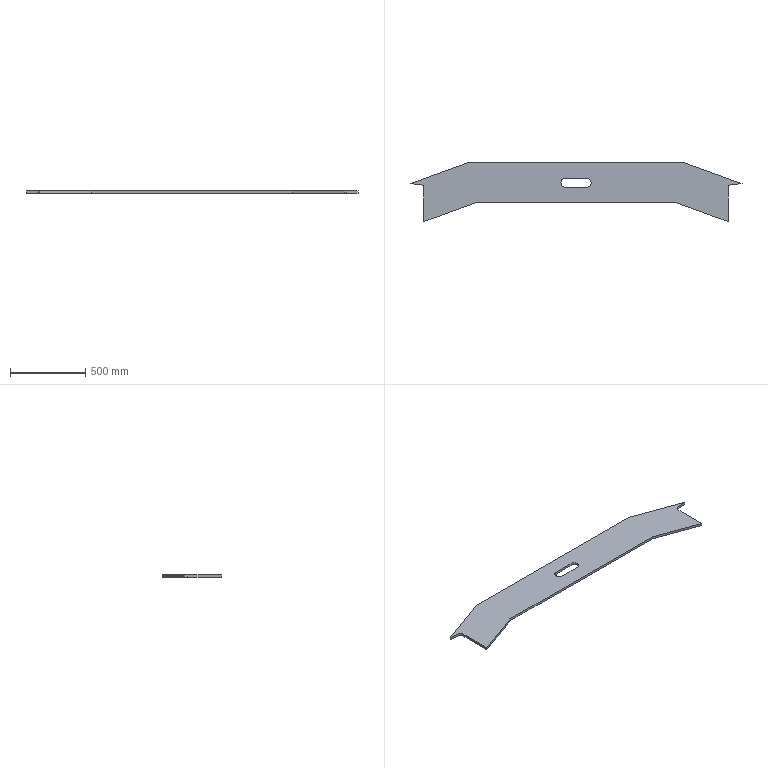Part | SolidWorks | features ICE 2, Fillet 1, FlatPattern 1, SMBaseFlange 1, SheetMetal 1 | 1 solid | 19 faces | box 2205 x 392.571 x 16 mm | volume 8722850 mm3 | plane 14 | cylinder 5 | commonest cylinder face diameters 60 x3 40 x2
STEP:
#1=CARTESIAN_POINT('',(-100.,-134.,0.));
#2=VERTEX_POINT('',#1);
#3=CARTESIAN_POINT('',(-70.,-104.,0.));
#4=VERTEX_POINT('',#3);
#5=CARTESIAN_POINT('',(-70.,-134.,0.));
#6=DIRECTION('',(0.,0.,-1.));
#7=DIRECTION('',(-1.,0.,0.));
#8=AXIS2_PLACEMENT_3D('',#5,#6,#7);
#9=CIRCLE('',#8,30.);
#10=EDGE_CURVE('',#2,#4,#9,.T.);
#11=ORIENTED_EDGE('',*,*,#10,.F.);
#12=CARTESIAN_POINT('',(-100.,-134.,-16.));
#13=VERTEX_POINT('',#12);
#14=CARTESIAN_POINT('',(-100.,-134.,0.));
#15=DIRECTION('',(0.,0.,-1.));
#16=VECTOR('',#15,1000.);
#17=LINE('',#14,#16);
#18=EDGE_CURVE('',#2,#13,#17,.T.);
#19=ORIENTED_EDGE('',*,*,#18,.T.);
#20=CARTESIAN_POINT('',(-70.,-104.,-16.));
#21=VERTEX_POINT('',#20);
#22=CARTESIAN_POINT('',(-70.,-134.,-16.));
#23=DIRECTION('',(0.,0.,-1.));
#24=DIRECTION('',(-1.,0.,0.));
#25=AXIS2_PLACEMENT_3D('',#22,#23,#24);
#26=CIRCLE('',#25,30.);
#27=EDGE_CURVE('',#13,#21,#26,.T.);
#28=ORIENTED_EDGE('',*,*,#27,.T.);
#29=CARTESIAN_POINT('',(-70.,-104.,0.));
#30=DIRECTION('',(0.,0.,-1.));
#31=VECTOR('',#30,1000.);
#32=LINE('',#29,#31);
#33=EDGE_CURVE('',#4,#21,#32,.T.);
#34=ORIENTED_EDGE('',*,*,#33,.F.);
#35=EDGE_LOOP('',(#11,#19,#28,#34));
#36=FACE_OUTER_BOUND('',#35,.T.);
#37=CARTESIAN_POINT('',(-70.,-134.,0.));
#38=DIRECTION('',(0.,0.,-1.));
#39=DIRECTION('',(-1.,0.,0.));
#40=AXIS2_PLACEMENT_3D('',#37,#38,#39);
#41=CYLINDRICAL_SURFACE('',#40,30.);
#42=ADVANCED_FACE('',(#36),#41,.F.);
#43=CARTESIAN_POINT('',(715.,0.,0.));
#44=VERTEX_POINT('',#43);
#45=CARTESIAN_POINT('',(-715.,0.,0.));
#46=VERTEX_POINT('',#45);
#47=CARTESIAN_POINT('',(-715.,0.,0.));
#48=DIRECTION('',(-1.,0.,0.));
#49=VECTOR('',#48,1000.);
#50=LINE('',#47,#49);
#51=EDGE_CURVE('',#44,#46,#50,.T.);
#52=ORIENTED_EDGE('',*,*,#51,.F.);
#53=CARTESIAN_POINT('',(715.,0.,-16.));
#54=VERTEX_POINT('',#53);
#55=CARTESIAN_POINT('',(715.,0.,-16.));
#56=DIRECTION('',(0.,0.,1.));
#57=VECTOR('',#56,1000.);
#58=LINE('',#55,#57);
#59=EDGE_CURVE('',#54,#44,#58,.T.);
#60=ORIENTED_EDGE('',*,*,#59,.F.);
#61=CARTESIAN_POINT('',(-715.,0.,-16.));
#62=VERTEX_POINT('',#61);
#63=CARTESIAN_POINT('',(-715.,0.,-16.));
#64=DIRECTION('',(-1.,0.,0.));
#65=VECTOR('',#64,1000.);
#66=LINE('',#63,#65);
#67=EDGE_CURVE('',#54,#62,#66,.T.);
#68=ORIENTED_EDGE('',*,*,#67,.T.);
#69=CARTESIAN_POINT('',(-715.,0.,-16.));
#70=DIRECTION('',(0.,0.,1.));
#71=VECTOR('',#70,1000.);
#72=LINE('',#69,#71);
#73=EDGE_CURVE('',#62,#46,#72,.T.);
#74=ORIENTED_EDGE('',*,*,#73,.T.);
#75=EDGE_LOOP('',(#52,#60,#68,#74));
#76=FACE_OUTER_BOUND('',#75,.T.);
#77=CARTESIAN_POINT('',(-715.,0.,-16.));
#78=DIRECTION('',(0.,1.,0.));
#79=DIRECTION('',(0.,0.,1.));
#80=AXIS2_PLACEMENT_3D('',#77,#78,#79);
#81=PLANE('',#80);
#82=ADVANCED_FACE('',(#76),#81,.T.);
#83=CARTESIAN_POINT('',(1102.619,-141.082,-16.));
#84=VERTEX_POINT('',#83);
#85=CARTESIAN_POINT('',(1102.619,-141.082,0.));
#86=VERTEX_POINT('',#85);
#87=CARTESIAN_POINT('',(1102.619,-141.082,-16.));
#88=DIRECTION('',(0.,0.,1.));
#89=VECTOR('',#88,1000.);
#90=LINE('',#87,#89);
#91=EDGE_CURVE('',#84,#86,#90,.T.);
#92=ORIENTED_EDGE('',*,*,#91,.F.);
#93=CARTESIAN_POINT('',(715.,0.,-16.));
#94=DIRECTION('',(-0.9397,0.342,0.));
#95=VECTOR('',#94,1000.);
#96=LINE('',#93,#95);
#97=EDGE_CURVE('',#84,#54,#96,.T.);
#98=ORIENTED_EDGE('',*,*,#97,.T.);
#99=ORIENTED_EDGE('',*,*,#59,.T.);
#100=CARTESIAN_POINT('',(715.,0.,0.));
#101=DIRECTION('',(-0.9397,0.342,0.));
#102=VECTOR('',#101,1000.);
#103=LINE('',#100,#102);
#104=EDGE_CURVE('',#86,#44,#103,.T.);
#105=ORIENTED_EDGE('',*,*,#104,.F.);
#106=EDGE_LOOP('',(#92,#98,#99,#105));
#107=FACE_OUTER_BOUND('',#106,.T.);
#108=CARTESIAN_POINT('',(715.,0.,-16.));
#109=DIRECTION('',(0.342,0.9397,0.));
#110=DIRECTION('',(-0.9397,0.342,0.));
#111=AXIS2_PLACEMENT_3D('',#108,#109,#110);
#112=PLANE('',#111);
#113=ADVANCED_FACE('',(#107),#112,.T.);
#114=CARTESIAN_POINT('',(1010.,-392.571,0.));
#115=VERTEX_POINT('',#114);
#116=CARTESIAN_POINT('',(1010.,-392.571,-16.));
#117=VERTEX_POINT('',#116);
#118=CARTESIAN_POINT('',(1010.,-392.571,-16.));
#119=DIRECTION('',(0.,0.,-1.));
#120=VECTOR('',#119,1000.);
#121=LINE('',#118,#120);
#122=EDGE_CURVE('',#115,#117,#121,.T.);
#123=ORIENTED_EDGE('',*,*,#122,.F.);
#124=CARTESIAN_POINT('',(667.744,-268.,0.));
#125=VERTEX_POINT('',#124);
#126=CARTESIAN_POINT('',(667.744,-268.,0.));
#127=DIRECTION('',(0.9397,-0.342,0.));
#128=VECTOR('',#127,1000.);
#129=LINE('',#126,#128);
#130=EDGE_CURVE('',#125,#115,#129,.T.);
#131=ORIENTED_EDGE('',*,*,#130,.F.);
#132=CARTESIAN_POINT('',(667.744,-268.,-16.));
#133=VERTEX_POINT('',#132);
#134=CARTESIAN_POINT('',(667.744,-268.,-16.));
#135=DIRECTION('',(0.,0.,1.));
#136=VECTOR('',#135,1000.);
#137=LINE('',#134,#136);
#138=EDGE_CURVE('',#133,#125,#137,.T.);
#139=ORIENTED_EDGE('',*,*,#138,.F.);
#140=CARTESIAN_POINT('',(667.744,-268.,-16.));
#141=DIRECTION('',(0.9397,-0.342,0.));
#142=VECTOR('',#141,1000.);
#143=LINE('',#140,#142);
#144=EDGE_CURVE('',#133,#117,#143,.T.);
#145=ORIENTED_EDGE('',*,*,#144,.T.);
#146=EDGE_LOOP('',(#123,#131,#139,#145));
#147=FACE_OUTER_BOUND('',#146,.T.);
#148=CARTESIAN_POINT('',(667.744,-268.,-16.));
#149=DIRECTION('',(-0.342,-0.9397,0.));
#150=DIRECTION('',(0.9397,-0.342,0.));
#151=AXIS2_PLACEMENT_3D('',#148,#149,#150);
#152=PLANE('',#151);
#153=ADVANCED_FACE('',(#147),#152,.T.);
#154=CARTESIAN_POINT('',(-667.744,-268.,0.));
#155=VERTEX_POINT('',#154);
#156=CARTESIAN_POINT('',(-667.744,-268.,0.));
#157=DIRECTION('',(1.,0.,0.));
#158=VECTOR('',#157,1000.);
#159=LINE('',#156,#158);
#160=EDGE_CURVE('',#155,#125,#159,.T.);
#161=ORIENTED_EDGE('',*,*,#160,.F.);
#162=CARTESIAN_POINT('',(-667.744,-268.,-16.));
#163=VERTEX_POINT('',#162);
#164=CARTESIAN_POINT('',(-667.744,-268.,-16.));
#165=DIRECTION('',(0.,0.,1.));
#166=VECTOR('',#165,1000.);
#167=LINE('',#164,#166);
#168=EDGE_CURVE('',#163,#155,#167,.T.);
#169=ORIENTED_EDGE('',*,*,#168,.F.);
#170=CARTESIAN_POINT('',(-667.744,-268.,-16.));
#171=DIRECTION('',(1.,0.,0.));
#172=VECTOR('',#171,1000.);
#173=LINE('',#170,#172);
#174=EDGE_CURVE('',#163,#133,#173,.T.);
#175=ORIENTED_EDGE('',*,*,#174,.T.);
#176=ORIENTED_EDGE('',*,*,#138,.T.);
#177=EDGE_LOOP('',(#161,#169,#175,#176));
#178=FACE_OUTER_BOUND('',#177,.T.);
#179=CARTESIAN_POINT('',(-667.744,-268.,-16.));
#180=DIRECTION('',(0.,-1.,0.));
#181=DIRECTION('',(0.,0.,-1.));
#182=AXIS2_PLACEMENT_3D('',#179,#180,#181);
#183=PLANE('',#182);
#184=ADVANCED_FACE('',(#178),#183,.T.);
#185=CARTESIAN_POINT('',(-1010.,-392.571,-16.));
#186=VERTEX_POINT('',#185);
#187=CARTESIAN_POINT('',(-1010.,-392.571,0.));
#188=VERTEX_POINT('',#187);
#189=CARTESIAN_POINT('',(-1010.,-392.571,-16.));
#190=DIRECTION('',(0.,0.,1.));
#191=VECTOR('',#190,1000.);
#192=LINE('',#189,#191);
#193=EDGE_CURVE('',#186,#188,#192,.T.);
#194=ORIENTED_EDGE('',*,*,#193,.F.);
#195=CARTESIAN_POINT('',(-667.744,-268.,-16.));
#196=DIRECTION('',(0.9397,0.342,0.));
#197=VECTOR('',#196,1000.);
#198=LINE('',#195,#197);
#199=EDGE_CURVE('',#186,#163,#198,.T.);
#200=ORIENTED_EDGE('',*,*,#199,.T.);
#201=ORIENTED_EDGE('',*,*,#168,.T.);
#202=CARTESIAN_POINT('',(-667.744,-268.,0.));
#203=DIRECTION('',(0.9397,0.342,0.));
#204=VECTOR('',#203,1000.);
#205=LINE('',#202,#204);
#206=EDGE_CURVE('',#188,#155,#205,.T.);
#207=ORIENTED_EDGE('',*,*,#206,.F.);
#208=EDGE_LOOP('',(#194,#200,#201,#207));
#209=FACE_OUTER_BOUND('',#208,.T.);
#210=CARTESIAN_POINT('',(-667.744,-268.,-16.));
#211=DIRECTION('',(0.342,-0.9397,0.));
#212=DIRECTION('',(0.9397,0.342,0.));
#213=AXIS2_PLACEMENT_3D('',#210,#211,#212);
#214=PLANE('',#213);
#215=ADVANCED_FACE('',(#209),#214,.T.);
#216=CARTESIAN_POINT('',(-1102.619,-141.082,0.));
#217=VERTEX_POINT('',#216);
#218=CARTESIAN_POINT('',(-1102.619,-141.082,-16.));
#219=VERTEX_POINT('',#218);
#220=CARTESIAN_POINT('',(-1102.619,-141.082,-16.));
#221=DIRECTION('',(0.,0.,-1.));
#222=VECTOR('',#221,1000.);
#223=LINE('',#220,#222);
#224=EDGE_CURVE('',#217,#219,#223,.T.);
#225=ORIENTED_EDGE('',*,*,#224,.F.);
#226=CARTESIAN_POINT('',(-715.,0.,0.));
#227=DIRECTION('',(-0.9397,-0.342,0.));
#228=VECTOR('',#227,1000.);
#229=LINE('',#226,#228);
#230=EDGE_CURVE('',#46,#217,#229,.T.);
#231=ORIENTED_EDGE('',*,*,#230,.F.);
#232=ORIENTED_EDGE('',*,*,#73,.F.);
#233=CARTESIAN_POINT('',(-715.,0.,-16.));
#234=DIRECTION('',(-0.9397,-0.342,0.));
#235=VECTOR('',#234,1000.);
#236=LINE('',#233,#235);
#237=EDGE_CURVE('',#62,#219,#236,.T.);
#238=ORIENTED_EDGE('',*,*,#237,.T.);
#239=EDGE_LOOP('',(#225,#231,#232,#238));
#240=FACE_OUTER_BOUND('',#239,.T.);
#241=CARTESIAN_POINT('',(-715.,0.,-16.));
#242=DIRECTION('',(-0.342,0.9397,0.));
#243=DIRECTION('',(-0.9397,-0.342,0.));
#244=AXIS2_PLACEMENT_3D('',#241,#242,#243);
#245=PLANE('',#244);
#246=ADVANCED_FACE('',(#240),#245,.T.);
#247=CARTESIAN_POINT('',(70.,-164.,-16.));
#248=VERTEX_POINT('',#247);
#249=CARTESIAN_POINT('',(-70.,-164.,-16.));
#250=VERTEX_POINT('',#249);
#251=CARTESIAN_POINT('',(70.,-164.,-16.));
#252=DIRECTION('',(-1.,0.,0.));
#253=VECTOR('',#252,1000.);
#254=LINE('',#251,#253);
#255=EDGE_CURVE('',#248,#250,#254,.T.);
#256=ORIENTED_EDGE('',*,*,#255,.F.);
#257=CARTESIAN_POINT('',(70.,-104.,-16.));
#258=VERTEX_POINT('',#257);
#259=CARTESIAN_POINT('',(70.,-134.,-16.));
#260=DIRECTION('',(0.,0.,-1.));
#261=DIRECTION('',(-1.,0.,0.));
#262=AXIS2_PLACEMENT_3D('',#259,#260,#261);
#263=CIRCLE('',#262,30.);
#264=EDGE_CURVE('',#258,#248,#263,.T.);
#265=ORIENTED_EDGE('',*,*,#264,.F.);
#266=CARTESIAN_POINT('',(70.,-104.,-16.));
#267=DIRECTION('',(1.,0.,0.));
#268=VECTOR('',#267,1000.);
#269=LINE('',#266,#268);
#270=EDGE_CURVE('',#21,#258,#269,.T.);
#271=ORIENTED_EDGE('',*,*,#270,.F.);
#272=ORIENTED_EDGE('',*,*,#27,.F.);
#273=CARTESIAN_POINT('',(-70.,-134.,-16.));
#274=DIRECTION('',(0.,0.,-1.));
#275=DIRECTION('',(-1.,0.,0.));
#276=AXIS2_PLACEMENT_3D('',#273,#274,#275);
#277=CIRCLE('',#276,30.);
#278=EDGE_CURVE('',#250,#13,#277,.T.);
#279=ORIENTED_EDGE('',*,*,#278,.F.);
#280=EDGE_LOOP('',(#256,#265,#271,#272,#279));
#281=FACE_BOUND('',#280,.T.);
#282=CARTESIAN_POINT('',(-1010.,-168.167,-16.));
#283=VERTEX_POINT('',#282);
#284=CARTESIAN_POINT('',(-1010.,-150.,-16.));
#285=DIRECTION('',(0.,1.,0.));
#286=VECTOR('',#285,1000.);
#287=LINE('',#284,#286);
#288=EDGE_CURVE('',#186,#283,#287,.T.);
#289=ORIENTED_EDGE('',*,*,#288,.T.);
#290=CARTESIAN_POINT('',(-1028.083,-148.259,-16.));
#291=VERTEX_POINT('',#290);
#292=CARTESIAN_POINT('',(-1030.,-168.167,-16.));
#293=DIRECTION('',(0.,0.,1.));
#294=DIRECTION('',(1.,0.,0.));
#295=AXIS2_PLACEMENT_3D('',#292,#293,#294);
#296=CIRCLE('',#295,20.);
#297=EDGE_CURVE('',#283,#291,#296,.T.);
#298=ORIENTED_EDGE('',*,*,#297,.T.);
#299=CARTESIAN_POINT('',(-1310.,-121.113,-16.));
#300=DIRECTION('',(-0.9954,0.09585,0.));
#301=VECTOR('',#300,1000.);
#302=LINE('',#299,#301);
#303=EDGE_CURVE('',#291,#219,#302,.T.);
#304=ORIENTED_EDGE('',*,*,#303,.T.);
#305=ORIENTED_EDGE('',*,*,#237,.F.);
#306=ORIENTED_EDGE('',*,*,#67,.F.);
#307=ORIENTED_EDGE('',*,*,#97,.F.);
#308=CARTESIAN_POINT('',(1028.083,-148.259,-16.));
#309=VERTEX_POINT('',#308);
#310=CARTESIAN_POINT('',(1310.,-121.113,-16.));
#311=DIRECTION('',(-0.9954,-0.09585,0.));
#312=VECTOR('',#311,1000.);
#313=LINE('',#310,#312);
#314=EDGE_CURVE('',#84,#309,#313,.T.);
#315=ORIENTED_EDGE('',*,*,#314,.T.);
#316=CARTESIAN_POINT('',(1010.,-168.167,-16.));
#317=VERTEX_POINT('',#316);
#318=CARTESIAN_POINT('',(1030.,-168.167,-16.));
#319=DIRECTION('',(0.,0.,1.));
#320=DIRECTION('',(1.,0.,0.));
#321=AXIS2_PLACEMENT_3D('',#318,#319,#320);
#322=CIRCLE('',#321,20.);
#323=EDGE_CURVE('',#309,#317,#322,.T.);
#324=ORIENTED_EDGE('',*,*,#323,.T.);
#325=CARTESIAN_POINT('',(1010.,-150.,-16.));
#326=DIRECTION('',(0.,-1.,0.));
#327=VECTOR('',#326,1000.);
#328=LINE('',#325,#327);
#329=EDGE_CURVE('',#317,#117,#328,.T.);
#330=ORIENTED_EDGE('',*,*,#329,.T.);
#331=ORIENTED_EDGE('',*,*,#144,.F.);
#332=ORIENTED_EDGE('',*,*,#174,.F.);
#333=ORIENTED_EDGE('',*,*,#199,.F.);
#334=EDGE_LOOP('',(#289,#298,#304,#305,#306,#307,#315,#324,#330,#331,#332,#333));
#335=FACE_OUTER_BOUND('',#334,.T.);
#336=CARTESIAN_POINT('',(0.,0.,-16.));
#337=DIRECTION('',(0.,0.,1.));
#338=DIRECTION('',(1.,0.,0.));
#339=AXIS2_PLACEMENT_3D('',#336,#337,#338);
#340=PLANE('',#339);
#341=ADVANCED_FACE('',(#281,#335),#340,.F.);
#342=CARTESIAN_POINT('',(70.,-104.,0.));
#343=VERTEX_POINT('',#342);
#344=CARTESIAN_POINT('',(70.,-164.,0.));
#345=VERTEX_POINT('',#344);
#346=CARTESIAN_POINT('',(70.,-134.,0.));
#347=DIRECTION('',(0.,0.,-1.));
#348=DIRECTION('',(-1.,0.,0.));
#349=AXIS2_PLACEMENT_3D('',#346,#347,#348);
#350=CIRCLE('',#349,30.);
#351=EDGE_CURVE('',#343,#345,#350,.T.);
#352=ORIENTED_EDGE('',*,*,#351,.T.);
#353=CARTESIAN_POINT('',(-70.,-164.,0.));
#354=VERTEX_POINT('',#353);
#355=CARTESIAN_POINT('',(70.,-164.,0.));
#356=DIRECTION('',(-1.,0.,0.));
#357=VECTOR('',#356,1000.);
#358=LINE('',#355,#357);
#359=EDGE_CURVE('',#345,#354,#358,.T.);
#360=ORIENTED_EDGE('',*,*,#359,.T.);
#361=CARTESIAN_POINT('',(-70.,-134.,0.));
#362=DIRECTION('',(0.,0.,-1.));
#363=DIRECTION('',(-1.,0.,0.));
#364=AXIS2_PLACEMENT_3D('',#361,#362,#363);
#365=CIRCLE('',#364,30.);
#366=EDGE_CURVE('',#354,#2,#365,.T.);
#367=ORIENTED_EDGE('',*,*,#366,.T.);
#368=ORIENTED_EDGE('',*,*,#10,.T.);
#369=CARTESIAN_POINT('',(70.,-104.,0.));
#370=DIRECTION('',(1.,0.,0.));
#371=VECTOR('',#370,1000.);
#372=LINE('',#369,#371);
#373=EDGE_CURVE('',#4,#343,#372,.T.);
#374=ORIENTED_EDGE('',*,*,#373,.T.);
#375=EDGE_LOOP('',(#352,#360,#367,#368,#374));
#376=FACE_BOUND('',#375,.T.);
#377=CARTESIAN_POINT('',(-1028.083,-148.259,0.));
#378=VERTEX_POINT('',#377);
#379=CARTESIAN_POINT('',(-1310.,-121.113,0.));
#380=DIRECTION('',(-0.9954,0.09585,0.));
#381=VECTOR('',#380,1000.);
#382=LINE('',#379,#381);
#383=EDGE_CURVE('',#378,#217,#382,.T.);
#384=ORIENTED_EDGE('',*,*,#383,.F.);
#385=CARTESIAN_POINT('',(-1010.,-168.167,0.));
#386=VERTEX_POINT('',#385);
#387=CARTESIAN_POINT('',(-1030.,-168.167,0.));
#388=DIRECTION('',(0.,0.,-1.));
#389=DIRECTION('',(1.,0.,0.));
#390=AXIS2_PLACEMENT_3D('',#387,#388,#389);
#391=CIRCLE('',#390,20.);
#392=EDGE_CURVE('',#378,#386,#391,.T.);
#393=ORIENTED_EDGE('',*,*,#392,.T.);
#394=CARTESIAN_POINT('',(-1010.,0.,0.));
#395=DIRECTION('',(0.,1.,0.));
#396=VECTOR('',#395,1000.);
#397=LINE('',#394,#396);
#398=EDGE_CURVE('',#188,#386,#397,.T.);
#399=ORIENTED_EDGE('',*,*,#398,.F.);
#400=ORIENTED_EDGE('',*,*,#206,.T.);
#401=ORIENTED_EDGE('',*,*,#160,.T.);
#402=ORIENTED_EDGE('',*,*,#130,.T.);
#403=CARTESIAN_POINT('',(1010.,-168.167,0.));
#404=VERTEX_POINT('',#403);
#405=CARTESIAN_POINT('',(1010.,-150.,0.));
#406=DIRECTION('',(0.,-1.,0.));
#407=VECTOR('',#406,1000.);
#408=LINE('',#405,#407);
#409=EDGE_CURVE('',#404,#115,#408,.T.);
#410=ORIENTED_EDGE('',*,*,#409,.F.);
#411=CARTESIAN_POINT('',(1028.083,-148.259,0.));
#412=VERTEX_POINT('',#411);
#413=CARTESIAN_POINT('',(1030.,-168.167,0.));
#414=DIRECTION('',(0.,0.,-1.));
#415=DIRECTION('',(1.,0.,0.));
#416=AXIS2_PLACEMENT_3D('',#413,#414,#415);
#417=CIRCLE('',#416,20.);
#418=EDGE_CURVE('',#404,#412,#417,.T.);
#419=ORIENTED_EDGE('',*,*,#418,.T.);
#420=CARTESIAN_POINT('',(23.589,-244.981,0.));
#421=DIRECTION('',(-0.9954,-0.09585,0.));
#422=VECTOR('',#421,1000.);
#423=LINE('',#420,#422);
#424=EDGE_CURVE('',#86,#412,#423,.T.);
#425=ORIENTED_EDGE('',*,*,#424,.F.);
#426=ORIENTED_EDGE('',*,*,#104,.T.);
#427=ORIENTED_EDGE('',*,*,#51,.T.);
#428=ORIENTED_EDGE('',*,*,#230,.T.);
#429=EDGE_LOOP('',(#384,#393,#399,#400,#401,#402,#410,#419,#425,#426,#427,#428));
#430=FACE_OUTER_BOUND('',#429,.T.);
#431=CARTESIAN_POINT('',(0.,0.,0.));
#432=DIRECTION('',(0.,0.,1.));
#433=DIRECTION('',(1.,0.,0.));
#434=AXIS2_PLACEMENT_3D('',#431,#432,#433);
#435=PLANE('',#434);
#436=ADVANCED_FACE('',(#376,#430),#435,.T.);
#437=ORIENTED_EDGE('',*,*,#329,.F.);
#438=CARTESIAN_POINT('',(1010.,-168.167,0.));
#439=DIRECTION('',(0.,0.,1.));
#440=VECTOR('',#439,1000.);
#441=LINE('',#438,#440);
#442=EDGE_CURVE('',#317,#404,#441,.T.);
#443=ORIENTED_EDGE('',*,*,#442,.T.);
#444=ORIENTED_EDGE('',*,*,#409,.T.);
#445=ORIENTED_EDGE('',*,*,#122,.T.);
#446=EDGE_LOOP('',(#437,#443,#444,#445));
#447=FACE_OUTER_BOUND('',#446,.T.);
#448=CARTESIAN_POINT('',(1010.,-150.,-16.));
#449=DIRECTION('',(-1.,0.,0.));
#450=DIRECTION('',(0.,0.,1.));
#451=AXIS2_PLACEMENT_3D('',#448,#449,#450);
#452=PLANE('',#451);
#453=ADVANCED_FACE('',(#447),#452,.F.);
#454=ORIENTED_EDGE('',*,*,#424,.T.);
#455=CARTESIAN_POINT('',(1028.083,-148.259,-16.));
#456=DIRECTION('',(0.,0.,-1.));
#457=VECTOR('',#456,1000.);
#458=LINE('',#455,#457);
#459=EDGE_CURVE('',#412,#309,#458,.T.);
#460=ORIENTED_EDGE('',*,*,#459,.T.);
#461=ORIENTED_EDGE('',*,*,#314,.F.);
#462=ORIENTED_EDGE('',*,*,#91,.T.);
#463=EDGE_LOOP('',(#454,#460,#461,#462));
#464=FACE_OUTER_BOUND('',#463,.T.);
#465=CARTESIAN_POINT('',(1310.,-121.113,-16.));
#466=DIRECTION('',(-0.09585,0.9954,0.));
#467=DIRECTION('',(-0.9954,-0.09585,0.));
#468=AXIS2_PLACEMENT_3D('',#465,#466,#467);
#469=PLANE('',#468);
#470=ADVANCED_FACE('',(#464),#469,.F.);
#471=ORIENTED_EDGE('',*,*,#303,.F.);
#472=CARTESIAN_POINT('',(-1028.083,-148.259,0.));
#473=DIRECTION('',(0.,0.,1.));
#474=VECTOR('',#473,1000.);
#475=LINE('',#472,#474);
#476=EDGE_CURVE('',#291,#378,#475,.T.);
#477=ORIENTED_EDGE('',*,*,#476,.T.);
#478=ORIENTED_EDGE('',*,*,#383,.T.);
#479=ORIENTED_EDGE('',*,*,#224,.T.);
#480=EDGE_LOOP('',(#471,#477,#478,#479));
#481=FACE_OUTER_BOUND('',#480,.T.);
#482=CARTESIAN_POINT('',(-1310.,-121.113,-16.));
#483=DIRECTION('',(0.09585,0.9954,0.));
#484=DIRECTION('',(-0.9954,0.09585,0.));
#485=AXIS2_PLACEMENT_3D('',#482,#483,#484);
#486=PLANE('',#485);
#487=ADVANCED_FACE('',(#481),#486,.F.);
#488=ORIENTED_EDGE('',*,*,#398,.T.);
#489=CARTESIAN_POINT('',(-1010.,-168.167,-16.));
#490=DIRECTION('',(0.,0.,-1.));
#491=VECTOR('',#490,1000.);
#492=LINE('',#489,#491);
#493=EDGE_CURVE('',#386,#283,#492,.T.);
#494=ORIENTED_EDGE('',*,*,#493,.T.);
#495=ORIENTED_EDGE('',*,*,#288,.F.);
#496=ORIENTED_EDGE('',*,*,#193,.T.);
#497=EDGE_LOOP('',(#488,#494,#495,#496));
#498=FACE_OUTER_BOUND('',#497,.T.);
#499=CARTESIAN_POINT('',(-1010.,-150.,-16.));
#500=DIRECTION('',(1.,0.,0.));
#501=DIRECTION('',(0.,1.,0.));
#502=AXIS2_PLACEMENT_3D('',#499,#500,#501);
#503=PLANE('',#502);
#504=ADVANCED_FACE('',(#498),#503,.F.);
#505=ORIENTED_EDGE('',*,*,#323,.F.);
#506=ORIENTED_EDGE('',*,*,#459,.F.);
#507=ORIENTED_EDGE('',*,*,#418,.F.);
#508=ORIENTED_EDGE('',*,*,#442,.F.);
#509=EDGE_LOOP('',(#505,#506,#507,#508));
#510=FACE_OUTER_BOUND('',#509,.T.);
#511=CARTESIAN_POINT('',(1030.,-168.167,-16.));
#512=DIRECTION('',(0.,0.,-1.));
#513=DIRECTION('',(-1.,0.,0.));
#514=AXIS2_PLACEMENT_3D('',#511,#512,#513);
#515=CYLINDRICAL_SURFACE('',#514,20.);
#516=ADVANCED_FACE('',(#510),#515,.F.);
#517=ORIENTED_EDGE('',*,*,#297,.F.);
#518=ORIENTED_EDGE('',*,*,#493,.F.);
#519=ORIENTED_EDGE('',*,*,#392,.F.);
#520=ORIENTED_EDGE('',*,*,#476,.F.);
#521=EDGE_LOOP('',(#517,#518,#519,#520));
#522=FACE_OUTER_BOUND('',#521,.T.);
#523=CARTESIAN_POINT('',(-1030.,-168.167,-16.));
#524=DIRECTION('',(0.,0.,-1.));
#525=DIRECTION('',(-1.,0.,0.));
#526=AXIS2_PLACEMENT_3D('',#523,#524,#525);
#527=CYLINDRICAL_SURFACE('',#526,20.);
#528=ADVANCED_FACE('',(#522),#527,.F.);
#529=ORIENTED_EDGE('',*,*,#264,.T.);
#530=CARTESIAN_POINT('',(70.,-164.,0.));
#531=DIRECTION('',(0.,0.,-1.));
#532=VECTOR('',#531,1000.);
#533=LINE('',#530,#532);
#534=EDGE_CURVE('',#345,#248,#533,.T.);
#535=ORIENTED_EDGE('',*,*,#534,.F.);
#536=ORIENTED_EDGE('',*,*,#351,.F.);
#537=CARTESIAN_POINT('',(70.,-104.,0.));
#538=DIRECTION('',(0.,0.,-1.));
#539=VECTOR('',#538,1000.);
#540=LINE('',#537,#539);
#541=EDGE_CURVE('',#343,#258,#540,.T.);
#542=ORIENTED_EDGE('',*,*,#541,.T.);
#543=EDGE_LOOP('',(#529,#535,#536,#542));
#544=FACE_OUTER_BOUND('',#543,.T.);
#545=CARTESIAN_POINT('',(70.,-134.,0.));
#546=DIRECTION('',(0.,0.,-1.));
#547=DIRECTION('',(-1.,0.,0.));
#548=AXIS2_PLACEMENT_3D('',#545,#546,#547);
#549=CYLINDRICAL_SURFACE('',#548,30.);
#550=ADVANCED_FACE('',(#544),#549,.F.);
#551=ORIENTED_EDGE('',*,*,#270,.T.);
#552=ORIENTED_EDGE('',*,*,#541,.F.);
#553=ORIENTED_EDGE('',*,*,#373,.F.);
#554=ORIENTED_EDGE('',*,*,#33,.T.);
#555=EDGE_LOOP('',(#551,#552,#553,#554));
#556=FACE_OUTER_BOUND('',#555,.T.);
#557=CARTESIAN_POINT('',(70.,-104.,0.));
#558=DIRECTION('',(0.,1.,0.));
#559=DIRECTION('',(0.,0.,1.));
#560=AXIS2_PLACEMENT_3D('',#557,#558,#559);
#561=PLANE('',#560);
#562=ADVANCED_FACE('',(#556),#561,.F.);
#563=ORIENTED_EDGE('',*,*,#18,.F.);
#564=ORIENTED_EDGE('',*,*,#366,.F.);
#565=CARTESIAN_POINT('',(-70.,-164.,0.));
#566=DIRECTION('',(0.,0.,-1.));
#567=VECTOR('',#566,1000.);
#568=LINE('',#565,#567);
#569=EDGE_CURVE('',#354,#250,#568,.T.);
#570=ORIENTED_EDGE('',*,*,#569,.T.);
#571=ORIENTED_EDGE('',*,*,#278,.T.);
#572=EDGE_LOOP('',(#563,#564,#570,#571));
#573=FACE_OUTER_BOUND('',#572,.T.);
#574=CARTESIAN_POINT('',(-70.,-134.,0.));
#575=DIRECTION('',(0.,0.,-1.));
#576=DIRECTION('',(-1.,0.,0.));
#577=AXIS2_PLACEMENT_3D('',#574,#575,#576);
#578=CYLINDRICAL_SURFACE('',#577,30.);
#579=ADVANCED_FACE('',(#573),#578,.F.);
#580=ORIENTED_EDGE('',*,*,#255,.T.);
#581=ORIENTED_EDGE('',*,*,#569,.F.);
#582=ORIENTED_EDGE('',*,*,#359,.F.);
#583=ORIENTED_EDGE('',*,*,#534,.T.);
#584=EDGE_LOOP('',(#580,#581,#582,#583));
#585=FACE_OUTER_BOUND('',#584,.T.);
#586=CARTESIAN_POINT('',(70.,-164.,0.));
#587=DIRECTION('',(0.,-1.,0.));
#588=DIRECTION('',(1.,0.,0.));
#589=AXIS2_PLACEMENT_3D('',#586,#587,#588);
#590=PLANE('',#589);
#591=ADVANCED_FACE('',(#585),#590,.F.);
#592=CLOSED_SHELL('',(#42,#82,#113,#153,#184,#215,#246,#341,#436,#453,#470,#487,#504,#516,#528,#550,#562,#579,#591));
#593=MANIFOLD_SOLID_BREP('',#592);
#594=CARTESIAN_POINT('',(0.,0.,0.));
#595=DIRECTION('',(0.,0.,1.));
#596=DIRECTION('',(1.,0.,0.));
#597=AXIS2_PLACEMENT_3D('',#594,#595,#596);
#598=(LENGTH_UNIT()NAMED_UNIT(*)SI_UNIT(.MILLI.,.METRE.));
#599=UNCERTAINTY_MEASURE_WITH_UNIT(LENGTH_MEASURE(0.00001),#598,'','');
#600=(NAMED_UNIT(*)PLANE_ANGLE_UNIT()SI_UNIT($,.RADIAN.));
#601=(NAMED_UNIT(*)SI_UNIT($,.STERADIAN.)SOLID_ANGLE_UNIT());
#602=(GEOMETRIC_REPRESENTATION_CONTEXT(3)GLOBAL_UNCERTAINTY_ASSIGNED_CONTEXT((#599))GLOBAL_UNIT_ASSIGNED_CONTEXT((#598,#600,#601))REPRESENTATION_CONTEXT('',''));
#603=ADVANCED_BREP_SHAPE_REPRESENTATION('',(#593,#597),#602);